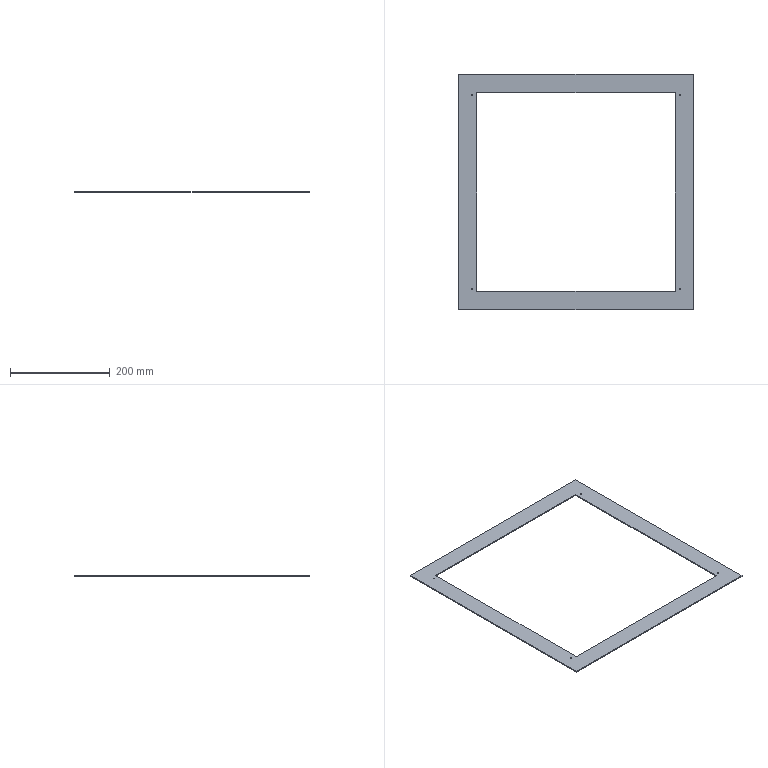Part | STEP file | Control Box Inner Spacer | 1 solid | 18 faces | box 470.879 x 472 x 2 mm | volume 126938 mm3 | plane 10 | cylinder 8 | commonest cylinder face diameters 3.2 x8
STEP:
#1=CARTESIAN_POINT('',(-1.097,-25.867,-2.));
#2=VERTEX_POINT('',#1);
#3=CARTESIAN_POINT('',(-4.297,-25.867,-2.));
#4=VERTEX_POINT('',#3);
#5=CARTESIAN_POINT('',(-2.697,-25.867,-2.));
#6=DIRECTION('',(0.,0.,-1.));
#7=DIRECTION('',(1.,0.,0.));
#8=AXIS2_PLACEMENT_3D('',#5,#6,#7);
#9=CIRCLE('',#8,1.6);
#10=EDGE_CURVE('',#2,#4,#9,.T.);
#11=ORIENTED_EDGE('',*,*,#10,.T.);
#12=CARTESIAN_POINT('',(-4.297,-25.867,0.));
#13=VERTEX_POINT('',#12);
#14=CARTESIAN_POINT('',(-4.297,-25.867,-2.));
#15=DIRECTION('',(0.,0.,1.));
#16=VECTOR('',#15,1000.);
#17=LINE('',#14,#16);
#18=EDGE_CURVE('',#4,#13,#17,.T.);
#19=ORIENTED_EDGE('',*,*,#18,.T.);
#20=CARTESIAN_POINT('',(-1.097,-25.867,0.));
#21=VERTEX_POINT('',#20);
#22=CARTESIAN_POINT('',(-2.697,-25.867,0.));
#23=DIRECTION('',(0.,0.,-1.));
#24=DIRECTION('',(1.,0.,0.));
#25=AXIS2_PLACEMENT_3D('',#22,#23,#24);
#26=CIRCLE('',#25,1.6);
#27=EDGE_CURVE('',#21,#13,#26,.T.);
#28=ORIENTED_EDGE('',*,*,#27,.F.);
#29=CARTESIAN_POINT('',(-1.097,-25.867,-2.));
#30=DIRECTION('',(0.,0.,1.));
#31=VECTOR('',#30,1000.);
#32=LINE('',#29,#31);
#33=EDGE_CURVE('',#2,#21,#32,.T.);
#34=ORIENTED_EDGE('',*,*,#33,.F.);
#35=EDGE_LOOP('',(#11,#19,#28,#34));
#36=FACE_OUTER_BOUND('',#35,.T.);
#37=CARTESIAN_POINT('',(-2.697,-25.867,-2.));
#38=DIRECTION('',(0.,0.,1.));
#39=DIRECTION('',(1.,0.,0.));
#40=AXIS2_PLACEMENT_3D('',#37,#38,#39);
#41=CYLINDRICAL_SURFACE('',#40,1.6);
#42=ADVANCED_FACE('',(#36),#41,.F.);
#43=CARTESIAN_POINT('',(-1.097,-414.867,-2.));
#44=VERTEX_POINT('',#43);
#45=CARTESIAN_POINT('',(-4.297,-414.867,-2.));
#46=VERTEX_POINT('',#45);
#47=CARTESIAN_POINT('',(-2.697,-414.867,-2.));
#48=DIRECTION('',(0.,0.,-1.));
#49=DIRECTION('',(1.,0.,0.));
#50=AXIS2_PLACEMENT_3D('',#47,#48,#49);
#51=CIRCLE('',#50,1.6);
#52=EDGE_CURVE('',#44,#46,#51,.T.);
#53=ORIENTED_EDGE('',*,*,#52,.T.);
#54=CARTESIAN_POINT('',(-4.297,-414.867,0.));
#55=VERTEX_POINT('',#54);
#56=CARTESIAN_POINT('',(-4.297,-414.867,-2.));
#57=DIRECTION('',(0.,0.,1.));
#58=VECTOR('',#57,1000.);
#59=LINE('',#56,#58);
#60=EDGE_CURVE('',#46,#55,#59,.T.);
#61=ORIENTED_EDGE('',*,*,#60,.T.);
#62=CARTESIAN_POINT('',(-1.097,-414.867,0.));
#63=VERTEX_POINT('',#62);
#64=CARTESIAN_POINT('',(-2.697,-414.867,0.));
#65=DIRECTION('',(0.,0.,-1.));
#66=DIRECTION('',(1.,0.,0.));
#67=AXIS2_PLACEMENT_3D('',#64,#65,#66);
#68=CIRCLE('',#67,1.6);
#69=EDGE_CURVE('',#63,#55,#68,.T.);
#70=ORIENTED_EDGE('',*,*,#69,.F.);
#71=CARTESIAN_POINT('',(-1.097,-414.867,-2.));
#72=DIRECTION('',(0.,0.,1.));
#73=VECTOR('',#72,1000.);
#74=LINE('',#71,#73);
#75=EDGE_CURVE('',#44,#63,#74,.T.);
#76=ORIENTED_EDGE('',*,*,#75,.F.);
#77=EDGE_LOOP('',(#53,#61,#70,#76));
#78=FACE_OUTER_BOUND('',#77,.T.);
#79=CARTESIAN_POINT('',(-2.697,-414.867,-2.));
#80=DIRECTION('',(0.,0.,1.));
#81=DIRECTION('',(1.,0.,0.));
#82=AXIS2_PLACEMENT_3D('',#79,#80,#81);
#83=CYLINDRICAL_SURFACE('',#82,1.6);
#84=ADVANCED_FACE('',(#78),#83,.F.);
#85=CARTESIAN_POINT('',(416.782,-25.867,-2.));
#86=VERTEX_POINT('',#85);
#87=CARTESIAN_POINT('',(413.582,-25.867,-2.));
#88=VERTEX_POINT('',#87);
#89=CARTESIAN_POINT('',(415.182,-25.867,-2.));
#90=DIRECTION('',(0.,0.,-1.));
#91=DIRECTION('',(1.,0.,0.));
#92=AXIS2_PLACEMENT_3D('',#89,#90,#91);
#93=CIRCLE('',#92,1.6);
#94=EDGE_CURVE('',#86,#88,#93,.T.);
#95=ORIENTED_EDGE('',*,*,#94,.T.);
#96=CARTESIAN_POINT('',(413.582,-25.867,0.));
#97=VERTEX_POINT('',#96);
#98=CARTESIAN_POINT('',(413.582,-25.867,-2.));
#99=DIRECTION('',(0.,0.,1.));
#100=VECTOR('',#99,1000.);
#101=LINE('',#98,#100);
#102=EDGE_CURVE('',#88,#97,#101,.T.);
#103=ORIENTED_EDGE('',*,*,#102,.T.);
#104=CARTESIAN_POINT('',(416.782,-25.867,0.));
#105=VERTEX_POINT('',#104);
#106=CARTESIAN_POINT('',(415.182,-25.867,0.));
#107=DIRECTION('',(0.,0.,-1.));
#108=DIRECTION('',(1.,0.,0.));
#109=AXIS2_PLACEMENT_3D('',#106,#107,#108);
#110=CIRCLE('',#109,1.6);
#111=EDGE_CURVE('',#105,#97,#110,.T.);
#112=ORIENTED_EDGE('',*,*,#111,.F.);
#113=CARTESIAN_POINT('',(416.782,-25.867,-2.));
#114=DIRECTION('',(0.,0.,1.));
#115=VECTOR('',#114,1000.);
#116=LINE('',#113,#115);
#117=EDGE_CURVE('',#86,#105,#116,.T.);
#118=ORIENTED_EDGE('',*,*,#117,.F.);
#119=EDGE_LOOP('',(#95,#103,#112,#118));
#120=FACE_OUTER_BOUND('',#119,.T.);
#121=CARTESIAN_POINT('',(415.182,-25.867,-2.));
#122=DIRECTION('',(0.,0.,1.));
#123=DIRECTION('',(1.,0.,0.));
#124=AXIS2_PLACEMENT_3D('',#121,#122,#123);
#125=CYLINDRICAL_SURFACE('',#124,1.6);
#126=ADVANCED_FACE('',(#120),#125,.F.);
#127=CARTESIAN_POINT('',(416.782,-414.867,-2.));
#128=VERTEX_POINT('',#127);
#129=CARTESIAN_POINT('',(413.582,-414.867,-2.));
#130=VERTEX_POINT('',#129);
#131=CARTESIAN_POINT('',(415.182,-414.867,-2.));
#132=DIRECTION('',(0.,0.,-1.));
#133=DIRECTION('',(1.,0.,0.));
#134=AXIS2_PLACEMENT_3D('',#131,#132,#133);
#135=CIRCLE('',#134,1.6);
#136=EDGE_CURVE('',#128,#130,#135,.T.);
#137=ORIENTED_EDGE('',*,*,#136,.T.);
#138=CARTESIAN_POINT('',(413.582,-414.867,0.));
#139=VERTEX_POINT('',#138);
#140=CARTESIAN_POINT('',(413.582,-414.867,-2.));
#141=DIRECTION('',(0.,0.,1.));
#142=VECTOR('',#141,1000.);
#143=LINE('',#140,#142);
#144=EDGE_CURVE('',#130,#139,#143,.T.);
#145=ORIENTED_EDGE('',*,*,#144,.T.);
#146=CARTESIAN_POINT('',(416.782,-414.867,0.));
#147=VERTEX_POINT('',#146);
#148=CARTESIAN_POINT('',(415.182,-414.867,0.));
#149=DIRECTION('',(0.,0.,-1.));
#150=DIRECTION('',(1.,0.,0.));
#151=AXIS2_PLACEMENT_3D('',#148,#149,#150);
#152=CIRCLE('',#151,1.6);
#153=EDGE_CURVE('',#147,#139,#152,.T.);
#154=ORIENTED_EDGE('',*,*,#153,.F.);
#155=CARTESIAN_POINT('',(416.782,-414.867,-2.));
#156=DIRECTION('',(0.,0.,1.));
#157=VECTOR('',#156,1000.);
#158=LINE('',#155,#157);
#159=EDGE_CURVE('',#128,#147,#158,.T.);
#160=ORIENTED_EDGE('',*,*,#159,.F.);
#161=EDGE_LOOP('',(#137,#145,#154,#160));
#162=FACE_OUTER_BOUND('',#161,.T.);
#163=CARTESIAN_POINT('',(415.182,-414.867,-2.));
#164=DIRECTION('',(0.,0.,1.));
#165=DIRECTION('',(1.,0.,0.));
#166=AXIS2_PLACEMENT_3D('',#163,#164,#165);
#167=CYLINDRICAL_SURFACE('',#166,1.6);
#168=ADVANCED_FACE('',(#162),#167,.F.);
#169=CARTESIAN_POINT('',(441.682,-456.367,-2.));
#170=VERTEX_POINT('',#169);
#171=CARTESIAN_POINT('',(441.682,15.633,-2.));
#172=VERTEX_POINT('',#171);
#173=CARTESIAN_POINT('',(441.682,0.,-2.));
#174=DIRECTION('',(0.,1.,0.));
#175=VECTOR('',#174,1000.);
#176=LINE('',#173,#175);
#177=EDGE_CURVE('',#170,#172,#176,.T.);
#178=ORIENTED_EDGE('',*,*,#177,.F.);
#179=CARTESIAN_POINT('',(-29.197,-456.367,-2.));
#180=VERTEX_POINT('',#179);
#181=CARTESIAN_POINT('',(0.,-456.367,-2.));
#182=DIRECTION('',(1.,0.,0.));
#183=VECTOR('',#182,1000.);
#184=LINE('',#181,#183);
#185=EDGE_CURVE('',#180,#170,#184,.T.);
#186=ORIENTED_EDGE('',*,*,#185,.F.);
#187=CARTESIAN_POINT('',(-29.197,15.633,-2.));
#188=VERTEX_POINT('',#187);
#189=CARTESIAN_POINT('',(-29.197,0.,-2.));
#190=DIRECTION('',(0.,-1.,0.));
#191=VECTOR('',#190,1000.);
#192=LINE('',#189,#191);
#193=EDGE_CURVE('',#188,#180,#192,.T.);
#194=ORIENTED_EDGE('',*,*,#193,.F.);
#195=CARTESIAN_POINT('',(0.,15.633,-2.));
#196=DIRECTION('',(-1.,0.,0.));
#197=VECTOR('',#196,1000.);
#198=LINE('',#195,#197);
#199=EDGE_CURVE('',#172,#188,#198,.T.);
#200=ORIENTED_EDGE('',*,*,#199,.F.);
#201=EDGE_LOOP('',(#178,#186,#194,#200));
#202=FACE_OUTER_BOUND('',#201,.T.);
#203=CARTESIAN_POINT('',(7.303,-419.867,-2.));
#204=VERTEX_POINT('',#203);
#205=CARTESIAN_POINT('',(7.303,-20.867,-2.));
#206=VERTEX_POINT('',#205);
#207=CARTESIAN_POINT('',(7.303,0.,-2.));
#208=DIRECTION('',(0.,1.,0.));
#209=VECTOR('',#208,1000.);
#210=LINE('',#207,#209);
#211=EDGE_CURVE('',#204,#206,#210,.T.);
#212=ORIENTED_EDGE('',*,*,#211,.F.);
#213=CARTESIAN_POINT('',(405.182,-419.867,-2.));
#214=VERTEX_POINT('',#213);
#215=CARTESIAN_POINT('',(0.,-419.867,-2.));
#216=DIRECTION('',(-1.,0.,0.));
#217=VECTOR('',#216,1000.);
#218=LINE('',#215,#217);
#219=EDGE_CURVE('',#214,#204,#218,.T.);
#220=ORIENTED_EDGE('',*,*,#219,.F.);
#221=CARTESIAN_POINT('',(405.182,-20.867,-2.));
#222=VERTEX_POINT('',#221);
#223=CARTESIAN_POINT('',(405.182,0.,-2.));
#224=DIRECTION('',(0.,-1.,0.));
#225=VECTOR('',#224,1000.);
#226=LINE('',#223,#225);
#227=EDGE_CURVE('',#222,#214,#226,.T.);
#228=ORIENTED_EDGE('',*,*,#227,.F.);
#229=CARTESIAN_POINT('',(0.,-20.867,-2.));
#230=DIRECTION('',(1.,0.,0.));
#231=VECTOR('',#230,1000.);
#232=LINE('',#229,#231);
#233=EDGE_CURVE('',#206,#222,#232,.T.);
#234=ORIENTED_EDGE('',*,*,#233,.F.);
#235=EDGE_LOOP('',(#212,#220,#228,#234));
#236=FACE_BOUND('',#235,.T.);
#237=ORIENTED_EDGE('',*,*,#10,.F.);
#238=CARTESIAN_POINT('',(-2.697,-25.867,-2.));
#239=DIRECTION('',(0.,0.,-1.));
#240=DIRECTION('',(1.,0.,0.));
#241=AXIS2_PLACEMENT_3D('',#238,#239,#240);
#242=CIRCLE('',#241,1.6);
#243=EDGE_CURVE('',#4,#2,#242,.T.);
#244=ORIENTED_EDGE('',*,*,#243,.F.);
#245=EDGE_LOOP('',(#237,#244));
#246=FACE_BOUND('',#245,.T.);
#247=ORIENTED_EDGE('',*,*,#52,.F.);
#248=CARTESIAN_POINT('',(-2.697,-414.867,-2.));
#249=DIRECTION('',(0.,0.,-1.));
#250=DIRECTION('',(1.,0.,0.));
#251=AXIS2_PLACEMENT_3D('',#248,#249,#250);
#252=CIRCLE('',#251,1.6);
#253=EDGE_CURVE('',#46,#44,#252,.T.);
#254=ORIENTED_EDGE('',*,*,#253,.F.);
#255=EDGE_LOOP('',(#247,#254));
#256=FACE_BOUND('',#255,.T.);
#257=ORIENTED_EDGE('',*,*,#94,.F.);
#258=CARTESIAN_POINT('',(415.182,-25.867,-2.));
#259=DIRECTION('',(0.,0.,-1.));
#260=DIRECTION('',(1.,0.,0.));
#261=AXIS2_PLACEMENT_3D('',#258,#259,#260);
#262=CIRCLE('',#261,1.6);
#263=EDGE_CURVE('',#88,#86,#262,.T.);
#264=ORIENTED_EDGE('',*,*,#263,.F.);
#265=EDGE_LOOP('',(#257,#264));
#266=FACE_BOUND('',#265,.T.);
#267=ORIENTED_EDGE('',*,*,#136,.F.);
#268=CARTESIAN_POINT('',(415.182,-414.867,-2.));
#269=DIRECTION('',(0.,0.,-1.));
#270=DIRECTION('',(1.,0.,0.));
#271=AXIS2_PLACEMENT_3D('',#268,#269,#270);
#272=CIRCLE('',#271,1.6);
#273=EDGE_CURVE('',#130,#128,#272,.T.);
#274=ORIENTED_EDGE('',*,*,#273,.F.);
#275=EDGE_LOOP('',(#267,#274));
#276=FACE_BOUND('',#275,.T.);
#277=CARTESIAN_POINT('',(0.,0.,-2.));
#278=DIRECTION('',(0.,0.,1.));
#279=DIRECTION('',(1.,0.,0.));
#280=AXIS2_PLACEMENT_3D('',#277,#278,#279);
#281=PLANE('',#280);
#282=ADVANCED_FACE('',(#202,#236,#246,#256,#266,#276),#281,.F.);
#283=ORIENTED_EDGE('',*,*,#199,.T.);
#284=CARTESIAN_POINT('',(-29.197,15.633,0.));
#285=VERTEX_POINT('',#284);
#286=CARTESIAN_POINT('',(-29.197,15.633,-2.));
#287=DIRECTION('',(0.,0.,1.));
#288=VECTOR('',#287,1000.);
#289=LINE('',#286,#288);
#290=EDGE_CURVE('',#188,#285,#289,.T.);
#291=ORIENTED_EDGE('',*,*,#290,.T.);
#292=CARTESIAN_POINT('',(441.682,15.633,0.));
#293=VERTEX_POINT('',#292);
#294=CARTESIAN_POINT('',(441.682,15.633,0.));
#295=DIRECTION('',(1.,0.,0.));
#296=VECTOR('',#295,1000.);
#297=LINE('',#294,#296);
#298=EDGE_CURVE('',#285,#293,#297,.T.);
#299=ORIENTED_EDGE('',*,*,#298,.T.);
#300=CARTESIAN_POINT('',(441.682,15.633,-2.));
#301=DIRECTION('',(0.,0.,-1.));
#302=VECTOR('',#301,1000.);
#303=LINE('',#300,#302);
#304=EDGE_CURVE('',#293,#172,#303,.T.);
#305=ORIENTED_EDGE('',*,*,#304,.T.);
#306=EDGE_LOOP('',(#283,#291,#299,#305));
#307=FACE_OUTER_BOUND('',#306,.T.);
#308=CARTESIAN_POINT('',(441.682,15.633,-2.));
#309=DIRECTION('',(0.,1.,0.));
#310=DIRECTION('',(-1.,0.,0.));
#311=AXIS2_PLACEMENT_3D('',#308,#309,#310);
#312=PLANE('',#311);
#313=ADVANCED_FACE('',(#307),#312,.T.);
#314=ORIENTED_EDGE('',*,*,#177,.T.);
#315=ORIENTED_EDGE('',*,*,#304,.F.);
#316=CARTESIAN_POINT('',(441.682,-456.367,0.));
#317=VERTEX_POINT('',#316);
#318=CARTESIAN_POINT('',(441.682,-456.367,0.));
#319=DIRECTION('',(0.,-1.,0.));
#320=VECTOR('',#319,1000.);
#321=LINE('',#318,#320);
#322=EDGE_CURVE('',#293,#317,#321,.T.);
#323=ORIENTED_EDGE('',*,*,#322,.T.);
#324=CARTESIAN_POINT('',(441.682,-456.367,-2.));
#325=DIRECTION('',(0.,0.,-1.));
#326=VECTOR('',#325,1000.);
#327=LINE('',#324,#326);
#328=EDGE_CURVE('',#317,#170,#327,.T.);
#329=ORIENTED_EDGE('',*,*,#328,.T.);
#330=EDGE_LOOP('',(#314,#315,#323,#329));
#331=FACE_OUTER_BOUND('',#330,.T.);
#332=CARTESIAN_POINT('',(441.682,-456.367,-2.));
#333=DIRECTION('',(1.,0.,0.));
#334=DIRECTION('',(0.,0.,-1.));
#335=AXIS2_PLACEMENT_3D('',#332,#333,#334);
#336=PLANE('',#335);
#337=ADVANCED_FACE('',(#331),#336,.T.);
#338=ORIENTED_EDGE('',*,*,#185,.T.);
#339=ORIENTED_EDGE('',*,*,#328,.F.);
#340=CARTESIAN_POINT('',(-29.197,-456.367,0.));
#341=VERTEX_POINT('',#340);
#342=CARTESIAN_POINT('',(-29.197,-456.367,0.));
#343=DIRECTION('',(-1.,0.,0.));
#344=VECTOR('',#343,1000.);
#345=LINE('',#342,#344);
#346=EDGE_CURVE('',#317,#341,#345,.T.);
#347=ORIENTED_EDGE('',*,*,#346,.T.);
#348=CARTESIAN_POINT('',(-29.197,-456.367,-2.));
#349=DIRECTION('',(0.,0.,-1.));
#350=VECTOR('',#349,1000.);
#351=LINE('',#348,#350);
#352=EDGE_CURVE('',#341,#180,#351,.T.);
#353=ORIENTED_EDGE('',*,*,#352,.T.);
#354=EDGE_LOOP('',(#338,#339,#347,#353));
#355=FACE_OUTER_BOUND('',#354,.T.);
#356=CARTESIAN_POINT('',(-29.197,-456.367,-2.));
#357=DIRECTION('',(0.,-1.,0.));
#358=DIRECTION('',(1.,0.,0.));
#359=AXIS2_PLACEMENT_3D('',#356,#357,#358);
#360=PLANE('',#359);
#361=ADVANCED_FACE('',(#355),#360,.T.);
#362=ORIENTED_EDGE('',*,*,#193,.T.);
#363=ORIENTED_EDGE('',*,*,#352,.F.);
#364=CARTESIAN_POINT('',(-29.197,15.633,0.));
#365=DIRECTION('',(0.,1.,0.));
#366=VECTOR('',#365,1000.);
#367=LINE('',#364,#366);
#368=EDGE_CURVE('',#341,#285,#367,.T.);
#369=ORIENTED_EDGE('',*,*,#368,.T.);
#370=ORIENTED_EDGE('',*,*,#290,.F.);
#371=EDGE_LOOP('',(#362,#363,#369,#370));
#372=FACE_OUTER_BOUND('',#371,.T.);
#373=CARTESIAN_POINT('',(-29.197,15.633,-2.));
#374=DIRECTION('',(-1.,0.,0.));
#375=DIRECTION('',(0.,-1.,0.));
#376=AXIS2_PLACEMENT_3D('',#373,#374,#375);
#377=PLANE('',#376);
#378=ADVANCED_FACE('',(#372),#377,.T.);
#379=CARTESIAN_POINT('',(7.303,-20.867,0.));
#380=VERTEX_POINT('',#379);
#381=CARTESIAN_POINT('',(7.303,-20.867,-2.));
#382=DIRECTION('',(0.,0.,1.));
#383=VECTOR('',#382,1000.);
#384=LINE('',#381,#383);
#385=EDGE_CURVE('',#206,#380,#384,.T.);
#386=ORIENTED_EDGE('',*,*,#385,.F.);
#387=ORIENTED_EDGE('',*,*,#233,.T.);
#388=CARTESIAN_POINT('',(405.182,-20.867,0.));
#389=VERTEX_POINT('',#388);
#390=CARTESIAN_POINT('',(405.182,-20.867,-2.));
#391=DIRECTION('',(0.,0.,-1.));
#392=VECTOR('',#391,1000.);
#393=LINE('',#390,#392);
#394=EDGE_CURVE('',#389,#222,#393,.T.);
#395=ORIENTED_EDGE('',*,*,#394,.F.);
#396=CARTESIAN_POINT('',(7.303,-20.867,0.));
#397=DIRECTION('',(1.,0.,0.));
#398=VECTOR('',#397,1000.);
#399=LINE('',#396,#398);
#400=EDGE_CURVE('',#380,#389,#399,.T.);
#401=ORIENTED_EDGE('',*,*,#400,.F.);
#402=EDGE_LOOP('',(#386,#387,#395,#401));
#403=FACE_OUTER_BOUND('',#402,.T.);
#404=CARTESIAN_POINT('',(7.303,-20.867,-2.));
#405=DIRECTION('',(0.,1.,0.));
#406=DIRECTION('',(0.,0.,1.));
#407=AXIS2_PLACEMENT_3D('',#404,#405,#406);
#408=PLANE('',#407);
#409=ADVANCED_FACE('',(#403),#408,.F.);
#410=CARTESIAN_POINT('',(7.303,-419.867,0.));
#411=VERTEX_POINT('',#410);
#412=CARTESIAN_POINT('',(7.303,-419.867,-2.));
#413=DIRECTION('',(0.,0.,1.));
#414=VECTOR('',#413,1000.);
#415=LINE('',#412,#414);
#416=EDGE_CURVE('',#204,#411,#415,.T.);
#417=ORIENTED_EDGE('',*,*,#416,.F.);
#418=ORIENTED_EDGE('',*,*,#211,.T.);
#419=ORIENTED_EDGE('',*,*,#385,.T.);
#420=CARTESIAN_POINT('',(7.303,-20.867,0.));
#421=DIRECTION('',(0.,1.,0.));
#422=VECTOR('',#421,1000.);
#423=LINE('',#420,#422);
#424=EDGE_CURVE('',#411,#380,#423,.T.);
#425=ORIENTED_EDGE('',*,*,#424,.F.);
#426=EDGE_LOOP('',(#417,#418,#419,#425));
#427=FACE_OUTER_BOUND('',#426,.T.);
#428=CARTESIAN_POINT('',(7.303,-20.867,-2.));
#429=DIRECTION('',(-1.,0.,0.));
#430=DIRECTION('',(0.,0.,1.));
#431=AXIS2_PLACEMENT_3D('',#428,#429,#430);
#432=PLANE('',#431);
#433=ADVANCED_FACE('',(#427),#432,.F.);
#434=CARTESIAN_POINT('',(405.182,-419.867,0.));
#435=VERTEX_POINT('',#434);
#436=CARTESIAN_POINT('',(405.182,-419.867,-2.));
#437=DIRECTION('',(0.,0.,1.));
#438=VECTOR('',#437,1000.);
#439=LINE('',#436,#438);
#440=EDGE_CURVE('',#214,#435,#439,.T.);
#441=ORIENTED_EDGE('',*,*,#440,.F.);
#442=ORIENTED_EDGE('',*,*,#219,.T.);
#443=ORIENTED_EDGE('',*,*,#416,.T.);
#444=CARTESIAN_POINT('',(7.303,-419.867,0.));
#445=DIRECTION('',(-1.,0.,0.));
#446=VECTOR('',#445,1000.);
#447=LINE('',#444,#446);
#448=EDGE_CURVE('',#435,#411,#447,.T.);
#449=ORIENTED_EDGE('',*,*,#448,.F.);
#450=EDGE_LOOP('',(#441,#442,#443,#449));
#451=FACE_OUTER_BOUND('',#450,.T.);
#452=CARTESIAN_POINT('',(7.303,-419.867,-2.));
#453=DIRECTION('',(0.,-1.,0.));
#454=DIRECTION('',(0.,0.,-1.));
#455=AXIS2_PLACEMENT_3D('',#452,#453,#454);
#456=PLANE('',#455);
#457=ADVANCED_FACE('',(#451),#456,.F.);
#458=ORIENTED_EDGE('',*,*,#394,.T.);
#459=ORIENTED_EDGE('',*,*,#227,.T.);
#460=ORIENTED_EDGE('',*,*,#440,.T.);
#461=CARTESIAN_POINT('',(405.182,-419.867,0.));
#462=DIRECTION('',(0.,-1.,0.));
#463=VECTOR('',#462,1000.);
#464=LINE('',#461,#463);
#465=EDGE_CURVE('',#389,#435,#464,.T.);
#466=ORIENTED_EDGE('',*,*,#465,.F.);
#467=EDGE_LOOP('',(#458,#459,#460,#466));
#468=FACE_OUTER_BOUND('',#467,.T.);
#469=CARTESIAN_POINT('',(405.182,-419.867,-2.));
#470=DIRECTION('',(1.,0.,0.));
#471=DIRECTION('',(0.,1.,0.));
#472=AXIS2_PLACEMENT_3D('',#469,#470,#471);
#473=PLANE('',#472);
#474=ADVANCED_FACE('',(#468),#473,.F.);
#475=ORIENTED_EDGE('',*,*,#18,.F.);
#476=ORIENTED_EDGE('',*,*,#243,.T.);
#477=ORIENTED_EDGE('',*,*,#33,.T.);
#478=CARTESIAN_POINT('',(-2.697,-25.867,0.));
#479=DIRECTION('',(0.,0.,-1.));
#480=DIRECTION('',(1.,0.,0.));
#481=AXIS2_PLACEMENT_3D('',#478,#479,#480);
#482=CIRCLE('',#481,1.6);
#483=EDGE_CURVE('',#13,#21,#482,.T.);
#484=ORIENTED_EDGE('',*,*,#483,.F.);
#485=EDGE_LOOP('',(#475,#476,#477,#484));
#486=FACE_OUTER_BOUND('',#485,.T.);
#487=CARTESIAN_POINT('',(-2.697,-25.867,-2.));
#488=DIRECTION('',(0.,0.,1.));
#489=DIRECTION('',(1.,0.,0.));
#490=AXIS2_PLACEMENT_3D('',#487,#488,#489);
#491=CYLINDRICAL_SURFACE('',#490,1.6);
#492=ADVANCED_FACE('',(#486),#491,.F.);
#493=ORIENTED_EDGE('',*,*,#60,.F.);
#494=ORIENTED_EDGE('',*,*,#253,.T.);
#495=ORIENTED_EDGE('',*,*,#75,.T.);
#496=CARTESIAN_POINT('',(-2.697,-414.867,0.));
#497=DIRECTION('',(0.,0.,-1.));
#498=DIRECTION('',(1.,0.,0.));
#499=AXIS2_PLACEMENT_3D('',#496,#497,#498);
#500=CIRCLE('',#499,1.6);
#501=EDGE_CURVE('',#55,#63,#500,.T.);
#502=ORIENTED_EDGE('',*,*,#501,.F.);
#503=EDGE_LOOP('',(#493,#494,#495,#502));
#504=FACE_OUTER_BOUND('',#503,.T.);
#505=CARTESIAN_POINT('',(-2.697,-414.867,-2.));
#506=DIRECTION('',(0.,0.,1.));
#507=DIRECTION('',(1.,0.,0.));
#508=AXIS2_PLACEMENT_3D('',#505,#506,#507);
#509=CYLINDRICAL_SURFACE('',#508,1.6);
#510=ADVANCED_FACE('',(#504),#509,.F.);
#511=ORIENTED_EDGE('',*,*,#102,.F.);
#512=ORIENTED_EDGE('',*,*,#263,.T.);
#513=ORIENTED_EDGE('',*,*,#117,.T.);
#514=CARTESIAN_POINT('',(415.182,-25.867,0.));
#515=DIRECTION('',(0.,0.,-1.));
#516=DIRECTION('',(1.,0.,0.));
#517=AXIS2_PLACEMENT_3D('',#514,#515,#516);
#518=CIRCLE('',#517,1.6);
#519=EDGE_CURVE('',#97,#105,#518,.T.);
#520=ORIENTED_EDGE('',*,*,#519,.F.);
#521=EDGE_LOOP('',(#511,#512,#513,#520));
#522=FACE_OUTER_BOUND('',#521,.T.);
#523=CARTESIAN_POINT('',(415.182,-25.867,-2.));
#524=DIRECTION('',(0.,0.,1.));
#525=DIRECTION('',(1.,0.,0.));
#526=AXIS2_PLACEMENT_3D('',#523,#524,#525);
#527=CYLINDRICAL_SURFACE('',#526,1.6);
#528=ADVANCED_FACE('',(#522),#527,.F.);
#529=ORIENTED_EDGE('',*,*,#144,.F.);
#530=ORIENTED_EDGE('',*,*,#273,.T.);
#531=ORIENTED_EDGE('',*,*,#159,.T.);
#532=CARTESIAN_POINT('',(415.182,-414.867,0.));
#533=DIRECTION('',(0.,0.,-1.));
#534=DIRECTION('',(1.,0.,0.));
#535=AXIS2_PLACEMENT_3D('',#532,#533,#534);
#536=CIRCLE('',#535,1.6);
#537=EDGE_CURVE('',#139,#147,#536,.T.);
#538=ORIENTED_EDGE('',*,*,#537,.F.);
#539=EDGE_LOOP('',(#529,#530,#531,#538));
#540=FACE_OUTER_BOUND('',#539,.T.);
#541=CARTESIAN_POINT('',(415.182,-414.867,-2.));
#542=DIRECTION('',(0.,0.,1.));
#543=DIRECTION('',(1.,0.,0.));
#544=AXIS2_PLACEMENT_3D('',#541,#542,#543);
#545=CYLINDRICAL_SURFACE('',#544,1.6);
#546=ADVANCED_FACE('',(#540),#545,.F.);
#547=ORIENTED_EDGE('',*,*,#346,.F.);
#548=ORIENTED_EDGE('',*,*,#322,.F.);
#549=ORIENTED_EDGE('',*,*,#298,.F.);
#550=ORIENTED_EDGE('',*,*,#368,.F.);
#551=EDGE_LOOP('',(#547,#548,#549,#550));
#552=FACE_OUTER_BOUND('',#551,.T.);
#553=ORIENTED_EDGE('',*,*,#465,.T.);
#554=ORIENTED_EDGE('',*,*,#448,.T.);
#555=ORIENTED_EDGE('',*,*,#424,.T.);
#556=ORIENTED_EDGE('',*,*,#400,.T.);
#557=EDGE_LOOP('',(#553,#554,#555,#556));
#558=FACE_BOUND('',#557,.T.);
#559=ORIENTED_EDGE('',*,*,#27,.T.);
#560=ORIENTED_EDGE('',*,*,#483,.T.);
#561=EDGE_LOOP('',(#559,#560));
#562=FACE_BOUND('',#561,.T.);
#563=ORIENTED_EDGE('',*,*,#69,.T.);
#564=ORIENTED_EDGE('',*,*,#501,.T.);
#565=EDGE_LOOP('',(#563,#564));
#566=FACE_BOUND('',#565,.T.);
#567=ORIENTED_EDGE('',*,*,#111,.T.);
#568=ORIENTED_EDGE('',*,*,#519,.T.);
#569=EDGE_LOOP('',(#567,#568));
#570=FACE_BOUND('',#569,.T.);
#571=ORIENTED_EDGE('',*,*,#153,.T.);
#572=ORIENTED_EDGE('',*,*,#537,.T.);
#573=EDGE_LOOP('',(#571,#572));
#574=FACE_BOUND('',#573,.T.);
#575=CARTESIAN_POINT('',(0.,0.,0.));
#576=DIRECTION('',(0.,0.,1.));
#577=DIRECTION('',(1.,0.,0.));
#578=AXIS2_PLACEMENT_3D('',#575,#576,#577);
#579=PLANE('',#578);
#580=ADVANCED_FACE('',(#552,#558,#562,#566,#570,#574),#579,.T.);
#581=CLOSED_SHELL('',(#42,#84,#126,#168,#282,#313,#337,#361,#378,#409,#433,#457,#474,#492,#510,#528,#546,#580));
#582=MANIFOLD_SOLID_BREP('',#581);
#583=CARTESIAN_POINT('',(0.,0.,0.));
#584=DIRECTION('',(0.,0.,1.));
#585=DIRECTION('',(1.,0.,0.));
#586=AXIS2_PLACEMENT_3D('',#583,#584,#585);
#587=(LENGTH_UNIT()NAMED_UNIT(*)SI_UNIT(.MILLI.,.METRE.));
#588=UNCERTAINTY_MEASURE_WITH_UNIT(LENGTH_MEASURE(0.00001),#587,'','');
#589=(NAMED_UNIT(*)PLANE_ANGLE_UNIT()SI_UNIT($,.RADIAN.));
#590=(NAMED_UNIT(*)SI_UNIT($,.STERADIAN.)SOLID_ANGLE_UNIT());
#591=(GEOMETRIC_REPRESENTATION_CONTEXT(3)GLOBAL_UNCERTAINTY_ASSIGNED_CONTEXT((#588))GLOBAL_UNIT_ASSIGNED_CONTEXT((#587,#589,#590))REPRESENTATION_CONTEXT('',''));
#592=ADVANCED_BREP_SHAPE_REPRESENTATION('',(#582,#586),#591);